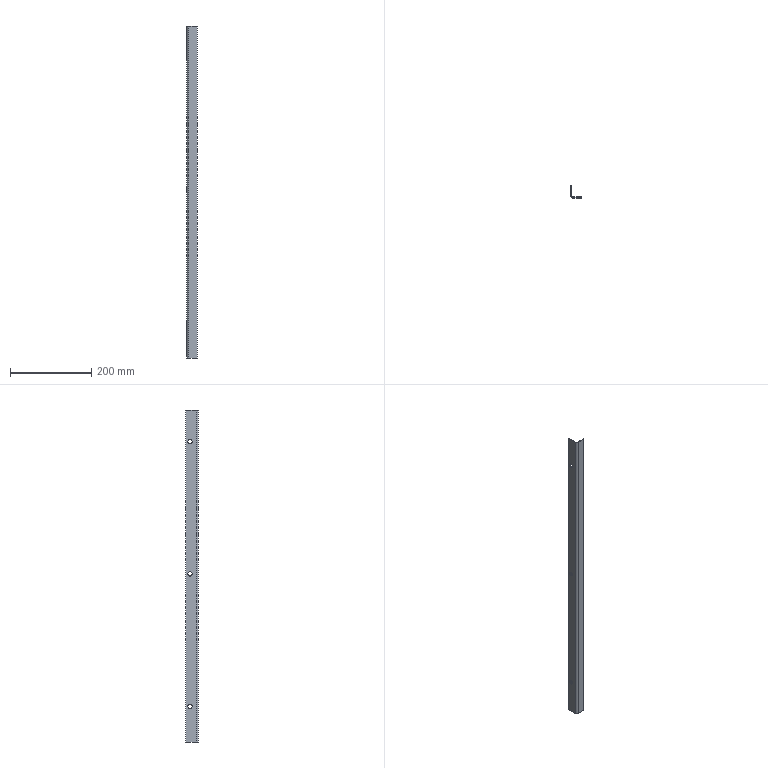Part | STEP file | 750038326 | 1 solid | 16 faces | box 25 x 30 x 815 mm | volume 103040 mm3 | cylinder 8 | plane 8 | commonest cylinder face diameters 10.5 x6 5 x1 10 x1
STEP:
#1=CARTESIAN_POINT('',(2.5,25.25,5.));
#2=VERTEX_POINT('',#1);
#3=CARTESIAN_POINT('',(2.5,14.75,5.));
#4=VERTEX_POINT('',#3);
#5=CARTESIAN_POINT('',(2.5,20.,5.));
#6=DIRECTION('',(-1.,0.,0.));
#7=DIRECTION('',(0.,-1.,0.));
#8=AXIS2_PLACEMENT_3D('',#5,#6,#7);
#9=CIRCLE('',#8,5.25);
#10=EDGE_CURVE('',#2,#4,#9,.T.);
#11=ORIENTED_EDGE('',*,*,#10,.F.);
#12=CARTESIAN_POINT('',(0.,25.25,5.));
#13=VERTEX_POINT('',#12);
#14=CARTESIAN_POINT('',(815.935,25.25,5.));
#15=DIRECTION('',(-1.,0.,0.));
#16=VECTOR('',#15,1000.);
#17=LINE('',#14,#16);
#18=EDGE_CURVE('',#2,#13,#17,.T.);
#19=ORIENTED_EDGE('',*,*,#18,.T.);
#20=CARTESIAN_POINT('',(0.,14.75,5.));
#21=VERTEX_POINT('',#20);
#22=CARTESIAN_POINT('',(0.,20.,5.));
#23=DIRECTION('',(1.,0.,0.));
#24=DIRECTION('',(0.,-1.,0.));
#25=AXIS2_PLACEMENT_3D('',#22,#23,#24);
#26=CIRCLE('',#25,5.25);
#27=EDGE_CURVE('',#21,#13,#26,.T.);
#28=ORIENTED_EDGE('',*,*,#27,.F.);
#29=CARTESIAN_POINT('',(815.935,14.75,5.));
#30=DIRECTION('',(-1.,0.,0.));
#31=VECTOR('',#30,1000.);
#32=LINE('',#29,#31);
#33=EDGE_CURVE('',#4,#21,#32,.T.);
#34=ORIENTED_EDGE('',*,*,#33,.F.);
#35=EDGE_LOOP('',(#11,#19,#28,#34));
#36=FACE_OUTER_BOUND('',#35,.T.);
#37=CARTESIAN_POINT('',(815.935,20.,5.));
#38=DIRECTION('',(-1.,0.,0.));
#39=DIRECTION('',(0.,-1.,0.));
#40=AXIS2_PLACEMENT_3D('',#37,#38,#39);
#41=CYLINDRICAL_SURFACE('',#40,5.25);
#42=ADVANCED_FACE('',(#36),#41,.F.);
#43=CARTESIAN_POINT('',(2.5,25.25,-320.));
#44=VERTEX_POINT('',#43);
#45=CARTESIAN_POINT('',(2.5,14.75,-320.));
#46=VERTEX_POINT('',#45);
#47=CARTESIAN_POINT('',(2.5,20.,-320.));
#48=DIRECTION('',(-1.,0.,0.));
#49=DIRECTION('',(0.,-1.,0.));
#50=AXIS2_PLACEMENT_3D('',#47,#48,#49);
#51=CIRCLE('',#50,5.25);
#52=EDGE_CURVE('',#44,#46,#51,.T.);
#53=ORIENTED_EDGE('',*,*,#52,.F.);
#54=CARTESIAN_POINT('',(0.,25.25,-320.));
#55=VERTEX_POINT('',#54);
#56=CARTESIAN_POINT('',(815.935,25.25,-320.));
#57=DIRECTION('',(-1.,0.,0.));
#58=VECTOR('',#57,1000.);
#59=LINE('',#56,#58);
#60=EDGE_CURVE('',#44,#55,#59,.T.);
#61=ORIENTED_EDGE('',*,*,#60,.T.);
#62=CARTESIAN_POINT('',(0.,14.75,-320.));
#63=VERTEX_POINT('',#62);
#64=CARTESIAN_POINT('',(0.,20.,-320.));
#65=DIRECTION('',(1.,0.,0.));
#66=DIRECTION('',(0.,-1.,0.));
#67=AXIS2_PLACEMENT_3D('',#64,#65,#66);
#68=CIRCLE('',#67,5.25);
#69=EDGE_CURVE('',#63,#55,#68,.T.);
#70=ORIENTED_EDGE('',*,*,#69,.F.);
#71=CARTESIAN_POINT('',(815.935,14.75,-320.));
#72=DIRECTION('',(-1.,0.,0.));
#73=VECTOR('',#72,1000.);
#74=LINE('',#71,#73);
#75=EDGE_CURVE('',#46,#63,#74,.T.);
#76=ORIENTED_EDGE('',*,*,#75,.F.);
#77=EDGE_LOOP('',(#53,#61,#70,#76));
#78=FACE_OUTER_BOUND('',#77,.T.);
#79=CARTESIAN_POINT('',(815.935,20.,-320.));
#80=DIRECTION('',(-1.,0.,0.));
#81=DIRECTION('',(0.,-1.,0.));
#82=AXIS2_PLACEMENT_3D('',#79,#80,#81);
#83=CYLINDRICAL_SURFACE('',#82,5.25);
#84=ADVANCED_FACE('',(#78),#83,.F.);
#85=CARTESIAN_POINT('',(2.5,25.25,330.));
#86=VERTEX_POINT('',#85);
#87=CARTESIAN_POINT('',(2.5,14.75,330.));
#88=VERTEX_POINT('',#87);
#89=CARTESIAN_POINT('',(2.5,20.,330.));
#90=DIRECTION('',(-1.,0.,0.));
#91=DIRECTION('',(0.,-1.,0.));
#92=AXIS2_PLACEMENT_3D('',#89,#90,#91);
#93=CIRCLE('',#92,5.25);
#94=EDGE_CURVE('',#86,#88,#93,.T.);
#95=ORIENTED_EDGE('',*,*,#94,.F.);
#96=CARTESIAN_POINT('',(0.,25.25,330.));
#97=VERTEX_POINT('',#96);
#98=CARTESIAN_POINT('',(815.935,25.25,330.));
#99=DIRECTION('',(-1.,0.,0.));
#100=VECTOR('',#99,1000.);
#101=LINE('',#98,#100);
#102=EDGE_CURVE('',#86,#97,#101,.T.);
#103=ORIENTED_EDGE('',*,*,#102,.T.);
#104=CARTESIAN_POINT('',(0.,14.75,330.));
#105=VERTEX_POINT('',#104);
#106=CARTESIAN_POINT('',(0.,20.,330.));
#107=DIRECTION('',(1.,0.,0.));
#108=DIRECTION('',(0.,-1.,0.));
#109=AXIS2_PLACEMENT_3D('',#106,#107,#108);
#110=CIRCLE('',#109,5.25);
#111=EDGE_CURVE('',#105,#97,#110,.T.);
#112=ORIENTED_EDGE('',*,*,#111,.F.);
#113=CARTESIAN_POINT('',(815.935,14.75,330.));
#114=DIRECTION('',(-1.,0.,0.));
#115=VECTOR('',#114,1000.);
#116=LINE('',#113,#115);
#117=EDGE_CURVE('',#88,#105,#116,.T.);
#118=ORIENTED_EDGE('',*,*,#117,.F.);
#119=EDGE_LOOP('',(#95,#103,#112,#118));
#120=FACE_OUTER_BOUND('',#119,.T.);
#121=CARTESIAN_POINT('',(815.935,20.,330.));
#122=DIRECTION('',(-1.,0.,0.));
#123=DIRECTION('',(0.,-1.,0.));
#124=AXIS2_PLACEMENT_3D('',#121,#122,#123);
#125=CYLINDRICAL_SURFACE('',#124,5.25);
#126=ADVANCED_FACE('',(#120),#125,.F.);
#127=CARTESIAN_POINT('',(0.,5.,407.5));
#128=VERTEX_POINT('',#127);
#129=CARTESIAN_POINT('',(0.,30.,407.5));
#130=VERTEX_POINT('',#129);
#131=CARTESIAN_POINT('',(0.,0.,407.5));
#132=DIRECTION('',(0.,1.,0.));
#133=VECTOR('',#132,1000.);
#134=LINE('',#131,#133);
#135=EDGE_CURVE('',#128,#130,#134,.T.);
#136=ORIENTED_EDGE('',*,*,#135,.T.);
#137=CARTESIAN_POINT('',(0.,30.,-407.5));
#138=VERTEX_POINT('',#137);
#139=CARTESIAN_POINT('',(0.,30.,407.5));
#140=DIRECTION('',(0.,0.,-1.));
#141=VECTOR('',#140,1000.);
#142=LINE('',#139,#141);
#143=EDGE_CURVE('',#130,#138,#142,.T.);
#144=ORIENTED_EDGE('',*,*,#143,.T.);
#145=CARTESIAN_POINT('',(0.,5.,-407.5));
#146=VERTEX_POINT('',#145);
#147=CARTESIAN_POINT('',(0.,0.,-407.5));
#148=DIRECTION('',(0.,-1.,0.));
#149=VECTOR('',#148,1000.);
#150=LINE('',#147,#149);
#151=EDGE_CURVE('',#138,#146,#150,.T.);
#152=ORIENTED_EDGE('',*,*,#151,.T.);
#153=CARTESIAN_POINT('',(0.,5.,407.5));
#154=DIRECTION('',(0.,0.,1.));
#155=VECTOR('',#154,1000.);
#156=LINE('',#153,#155);
#157=EDGE_CURVE('',#146,#128,#156,.T.);
#158=ORIENTED_EDGE('',*,*,#157,.T.);
#159=EDGE_LOOP('',(#136,#144,#152,#158));
#160=FACE_OUTER_BOUND('',#159,.T.);
#161=ORIENTED_EDGE('',*,*,#27,.T.);
#162=CARTESIAN_POINT('',(0.,20.,5.));
#163=DIRECTION('',(1.,0.,0.));
#164=DIRECTION('',(0.,-1.,0.));
#165=AXIS2_PLACEMENT_3D('',#162,#163,#164);
#166=CIRCLE('',#165,5.25);
#167=EDGE_CURVE('',#13,#21,#166,.T.);
#168=ORIENTED_EDGE('',*,*,#167,.T.);
#169=EDGE_LOOP('',(#161,#168));
#170=FACE_BOUND('',#169,.T.);
#171=ORIENTED_EDGE('',*,*,#69,.T.);
#172=CARTESIAN_POINT('',(0.,20.,-320.));
#173=DIRECTION('',(1.,0.,0.));
#174=DIRECTION('',(0.,-1.,0.));
#175=AXIS2_PLACEMENT_3D('',#172,#173,#174);
#176=CIRCLE('',#175,5.25);
#177=EDGE_CURVE('',#55,#63,#176,.T.);
#178=ORIENTED_EDGE('',*,*,#177,.T.);
#179=EDGE_LOOP('',(#171,#178));
#180=FACE_BOUND('',#179,.T.);
#181=ORIENTED_EDGE('',*,*,#111,.T.);
#182=CARTESIAN_POINT('',(0.,20.,330.));
#183=DIRECTION('',(1.,0.,0.));
#184=DIRECTION('',(0.,-1.,0.));
#185=AXIS2_PLACEMENT_3D('',#182,#183,#184);
#186=CIRCLE('',#185,5.25);
#187=EDGE_CURVE('',#97,#105,#186,.T.);
#188=ORIENTED_EDGE('',*,*,#187,.T.);
#189=EDGE_LOOP('',(#181,#188));
#190=FACE_BOUND('',#189,.T.);
#191=CARTESIAN_POINT('',(0.,0.,407.5));
#192=DIRECTION('',(-1.,0.,0.));
#193=DIRECTION('',(0.,-1.,0.));
#194=AXIS2_PLACEMENT_3D('',#191,#192,#193);
#195=PLANE('',#194);
#196=ADVANCED_FACE('',(#160,#170,#180,#190),#195,.T.);
#197=CARTESIAN_POINT('',(2.5,30.,-407.5));
#198=VERTEX_POINT('',#197);
#199=CARTESIAN_POINT('',(0.,30.,-407.5));
#200=DIRECTION('',(-1.,0.,0.));
#201=VECTOR('',#200,1000.);
#202=LINE('',#199,#201);
#203=EDGE_CURVE('',#198,#138,#202,.T.);
#204=ORIENTED_EDGE('',*,*,#203,.T.);
#205=ORIENTED_EDGE('',*,*,#143,.F.);
#206=CARTESIAN_POINT('',(2.5,30.,407.5));
#207=VERTEX_POINT('',#206);
#208=CARTESIAN_POINT('',(0.,30.,407.5));
#209=DIRECTION('',(1.,0.,0.));
#210=VECTOR('',#209,1000.);
#211=LINE('',#208,#210);
#212=EDGE_CURVE('',#130,#207,#211,.T.);
#213=ORIENTED_EDGE('',*,*,#212,.T.);
#214=CARTESIAN_POINT('',(2.5,30.,407.5));
#215=DIRECTION('',(0.,0.,-1.));
#216=VECTOR('',#215,1000.);
#217=LINE('',#214,#216);
#218=EDGE_CURVE('',#207,#198,#217,.T.);
#219=ORIENTED_EDGE('',*,*,#218,.T.);
#220=EDGE_LOOP('',(#204,#205,#213,#219));
#221=FACE_OUTER_BOUND('',#220,.T.);
#222=CARTESIAN_POINT('',(0.,30.,407.5));
#223=DIRECTION('',(0.,1.,0.));
#224=DIRECTION('',(-1.,0.,0.));
#225=AXIS2_PLACEMENT_3D('',#222,#223,#224);
#226=PLANE('',#225);
#227=ADVANCED_FACE('',(#221),#226,.T.);
#228=CARTESIAN_POINT('',(2.5,5.,407.5));
#229=VERTEX_POINT('',#228);
#230=CARTESIAN_POINT('',(2.5,0.,407.5));
#231=DIRECTION('',(0.,1.,0.));
#232=VECTOR('',#231,1000.);
#233=LINE('',#230,#232);
#234=EDGE_CURVE('',#229,#207,#233,.T.);
#235=ORIENTED_EDGE('',*,*,#234,.T.);
#236=ORIENTED_EDGE('',*,*,#212,.F.);
#237=ORIENTED_EDGE('',*,*,#135,.F.);
#238=CARTESIAN_POINT('',(5.,0.,407.5));
#239=VERTEX_POINT('',#238);
#240=CARTESIAN_POINT('',(5.,5.,407.5));
#241=DIRECTION('',(0.,0.,1.));
#242=DIRECTION('',(-1.,0.,0.));
#243=AXIS2_PLACEMENT_3D('',#240,#241,#242);
#244=CIRCLE('',#243,5.);
#245=EDGE_CURVE('',#128,#239,#244,.T.);
#246=ORIENTED_EDGE('',*,*,#245,.T.);
#247=CARTESIAN_POINT('',(25.,0.,407.5));
#248=VERTEX_POINT('',#247);
#249=CARTESIAN_POINT('',(0.,0.,407.5));
#250=DIRECTION('',(1.,0.,0.));
#251=VECTOR('',#250,1000.);
#252=LINE('',#249,#251);
#253=EDGE_CURVE('',#239,#248,#252,.T.);
#254=ORIENTED_EDGE('',*,*,#253,.T.);
#255=CARTESIAN_POINT('',(25.,2.5,407.5));
#256=VERTEX_POINT('',#255);
#257=CARTESIAN_POINT('',(25.,0.,407.5));
#258=DIRECTION('',(0.,1.,0.));
#259=VECTOR('',#258,1000.);
#260=LINE('',#257,#259);
#261=EDGE_CURVE('',#248,#256,#260,.T.);
#262=ORIENTED_EDGE('',*,*,#261,.T.);
#263=CARTESIAN_POINT('',(5.,2.5,407.5));
#264=VERTEX_POINT('',#263);
#265=CARTESIAN_POINT('',(0.,2.5,407.5));
#266=DIRECTION('',(-1.,0.,0.));
#267=VECTOR('',#266,1000.);
#268=LINE('',#265,#267);
#269=EDGE_CURVE('',#256,#264,#268,.T.);
#270=ORIENTED_EDGE('',*,*,#269,.T.);
#271=CARTESIAN_POINT('',(5.,5.,407.5));
#272=DIRECTION('',(0.,0.,-1.));
#273=DIRECTION('',(-1.,0.,0.));
#274=AXIS2_PLACEMENT_3D('',#271,#272,#273);
#275=CIRCLE('',#274,2.5);
#276=EDGE_CURVE('',#264,#229,#275,.T.);
#277=ORIENTED_EDGE('',*,*,#276,.T.);
#278=EDGE_LOOP('',(#235,#236,#237,#246,#254,#262,#270,#277));
#279=FACE_OUTER_BOUND('',#278,.T.);
#280=CARTESIAN_POINT('',(0.,0.,407.5));
#281=DIRECTION('',(0.,0.,1.));
#282=DIRECTION('',(1.,0.,0.));
#283=AXIS2_PLACEMENT_3D('',#280,#281,#282);
#284=PLANE('',#283);
#285=ADVANCED_FACE('',(#279),#284,.T.);
#286=ORIENTED_EDGE('',*,*,#245,.F.);
#287=ORIENTED_EDGE('',*,*,#157,.F.);
#288=CARTESIAN_POINT('',(5.,0.,-407.5));
#289=VERTEX_POINT('',#288);
#290=CARTESIAN_POINT('',(5.,5.,-407.5));
#291=DIRECTION('',(0.,0.,1.));
#292=DIRECTION('',(-1.,0.,0.));
#293=AXIS2_PLACEMENT_3D('',#290,#291,#292);
#294=CIRCLE('',#293,5.);
#295=EDGE_CURVE('',#146,#289,#294,.T.);
#296=ORIENTED_EDGE('',*,*,#295,.T.);
#297=CARTESIAN_POINT('',(5.,0.,407.5));
#298=DIRECTION('',(0.,0.,1.));
#299=VECTOR('',#298,1000.);
#300=LINE('',#297,#299);
#301=EDGE_CURVE('',#289,#239,#300,.T.);
#302=ORIENTED_EDGE('',*,*,#301,.T.);
#303=EDGE_LOOP('',(#286,#287,#296,#302));
#304=FACE_OUTER_BOUND('',#303,.T.);
#305=CARTESIAN_POINT('',(5.,5.,407.5));
#306=DIRECTION('',(0.,0.,-1.));
#307=DIRECTION('',(-1.,0.,0.));
#308=AXIS2_PLACEMENT_3D('',#305,#306,#307);
#309=CYLINDRICAL_SURFACE('',#308,5.);
#310=ADVANCED_FACE('',(#304),#309,.T.);
#311=ORIENTED_EDGE('',*,*,#295,.F.);
#312=ORIENTED_EDGE('',*,*,#151,.F.);
#313=ORIENTED_EDGE('',*,*,#203,.F.);
#314=CARTESIAN_POINT('',(2.5,5.,-407.5));
#315=VERTEX_POINT('',#314);
#316=CARTESIAN_POINT('',(2.5,0.,-407.5));
#317=DIRECTION('',(0.,1.,0.));
#318=VECTOR('',#317,1000.);
#319=LINE('',#316,#318);
#320=EDGE_CURVE('',#315,#198,#319,.T.);
#321=ORIENTED_EDGE('',*,*,#320,.F.);
#322=CARTESIAN_POINT('',(5.,2.5,-407.5));
#323=VERTEX_POINT('',#322);
#324=CARTESIAN_POINT('',(5.,5.,-407.5));
#325=DIRECTION('',(0.,0.,-1.));
#326=DIRECTION('',(-1.,0.,0.));
#327=AXIS2_PLACEMENT_3D('',#324,#325,#326);
#328=CIRCLE('',#327,2.5);
#329=EDGE_CURVE('',#323,#315,#328,.T.);
#330=ORIENTED_EDGE('',*,*,#329,.F.);
#331=CARTESIAN_POINT('',(25.,2.5,-407.5));
#332=VERTEX_POINT('',#331);
#333=CARTESIAN_POINT('',(25.,2.5,-407.5));
#334=DIRECTION('',(-1.,0.,0.));
#335=VECTOR('',#334,1000.);
#336=LINE('',#333,#335);
#337=EDGE_CURVE('',#332,#323,#336,.T.);
#338=ORIENTED_EDGE('',*,*,#337,.F.);
#339=CARTESIAN_POINT('',(25.,0.,-407.5));
#340=VERTEX_POINT('',#339);
#341=CARTESIAN_POINT('',(25.,0.,-407.5));
#342=DIRECTION('',(0.,1.,0.));
#343=VECTOR('',#342,1000.);
#344=LINE('',#341,#343);
#345=EDGE_CURVE('',#340,#332,#344,.T.);
#346=ORIENTED_EDGE('',*,*,#345,.F.);
#347=CARTESIAN_POINT('',(25.,0.,-407.5));
#348=DIRECTION('',(1.,0.,0.));
#349=VECTOR('',#348,1000.);
#350=LINE('',#347,#349);
#351=EDGE_CURVE('',#289,#340,#350,.T.);
#352=ORIENTED_EDGE('',*,*,#351,.F.);
#353=EDGE_LOOP('',(#311,#312,#313,#321,#330,#338,#346,#352));
#354=FACE_OUTER_BOUND('',#353,.T.);
#355=CARTESIAN_POINT('',(25.,0.,-407.5));
#356=DIRECTION('',(0.,0.,1.));
#357=DIRECTION('',(1.,0.,0.));
#358=AXIS2_PLACEMENT_3D('',#355,#356,#357);
#359=PLANE('',#358);
#360=ADVANCED_FACE('',(#354),#359,.F.);
#361=ORIENTED_EDGE('',*,*,#18,.F.);
#362=CARTESIAN_POINT('',(2.5,20.,5.));
#363=DIRECTION('',(-1.,0.,0.));
#364=DIRECTION('',(0.,-1.,0.));
#365=AXIS2_PLACEMENT_3D('',#362,#363,#364);
#366=CIRCLE('',#365,5.25);
#367=EDGE_CURVE('',#4,#2,#366,.T.);
#368=ORIENTED_EDGE('',*,*,#367,.F.);
#369=ORIENTED_EDGE('',*,*,#33,.T.);
#370=ORIENTED_EDGE('',*,*,#167,.F.);
#371=EDGE_LOOP('',(#361,#368,#369,#370));
#372=FACE_OUTER_BOUND('',#371,.T.);
#373=CARTESIAN_POINT('',(815.935,20.,5.));
#374=DIRECTION('',(-1.,0.,0.));
#375=DIRECTION('',(0.,-1.,0.));
#376=AXIS2_PLACEMENT_3D('',#373,#374,#375);
#377=CYLINDRICAL_SURFACE('',#376,5.25);
#378=ADVANCED_FACE('',(#372),#377,.F.);
#379=ORIENTED_EDGE('',*,*,#60,.F.);
#380=CARTESIAN_POINT('',(2.5,20.,-320.));
#381=DIRECTION('',(-1.,0.,0.));
#382=DIRECTION('',(0.,-1.,0.));
#383=AXIS2_PLACEMENT_3D('',#380,#381,#382);
#384=CIRCLE('',#383,5.25);
#385=EDGE_CURVE('',#46,#44,#384,.T.);
#386=ORIENTED_EDGE('',*,*,#385,.F.);
#387=ORIENTED_EDGE('',*,*,#75,.T.);
#388=ORIENTED_EDGE('',*,*,#177,.F.);
#389=EDGE_LOOP('',(#379,#386,#387,#388));
#390=FACE_OUTER_BOUND('',#389,.T.);
#391=CARTESIAN_POINT('',(815.935,20.,-320.));
#392=DIRECTION('',(-1.,0.,0.));
#393=DIRECTION('',(0.,-1.,0.));
#394=AXIS2_PLACEMENT_3D('',#391,#392,#393);
#395=CYLINDRICAL_SURFACE('',#394,5.25);
#396=ADVANCED_FACE('',(#390),#395,.F.);
#397=ORIENTED_EDGE('',*,*,#102,.F.);
#398=CARTESIAN_POINT('',(2.5,20.,330.));
#399=DIRECTION('',(-1.,0.,0.));
#400=DIRECTION('',(0.,-1.,0.));
#401=AXIS2_PLACEMENT_3D('',#398,#399,#400);
#402=CIRCLE('',#401,5.25);
#403=EDGE_CURVE('',#88,#86,#402,.T.);
#404=ORIENTED_EDGE('',*,*,#403,.F.);
#405=ORIENTED_EDGE('',*,*,#117,.T.);
#406=ORIENTED_EDGE('',*,*,#187,.F.);
#407=EDGE_LOOP('',(#397,#404,#405,#406));
#408=FACE_OUTER_BOUND('',#407,.T.);
#409=CARTESIAN_POINT('',(815.935,20.,330.));
#410=DIRECTION('',(-1.,0.,0.));
#411=DIRECTION('',(0.,-1.,0.));
#412=AXIS2_PLACEMENT_3D('',#409,#410,#411);
#413=CYLINDRICAL_SURFACE('',#412,5.25);
#414=ADVANCED_FACE('',(#408),#413,.F.);
#415=ORIENTED_EDGE('',*,*,#218,.F.);
#416=ORIENTED_EDGE('',*,*,#234,.F.);
#417=CARTESIAN_POINT('',(2.5,5.,407.5));
#418=DIRECTION('',(0.,0.,1.));
#419=VECTOR('',#418,1000.);
#420=LINE('',#417,#419);
#421=EDGE_CURVE('',#315,#229,#420,.T.);
#422=ORIENTED_EDGE('',*,*,#421,.F.);
#423=ORIENTED_EDGE('',*,*,#320,.T.);
#424=EDGE_LOOP('',(#415,#416,#422,#423));
#425=FACE_OUTER_BOUND('',#424,.T.);
#426=ORIENTED_EDGE('',*,*,#367,.T.);
#427=ORIENTED_EDGE('',*,*,#10,.T.);
#428=EDGE_LOOP('',(#426,#427));
#429=FACE_BOUND('',#428,.T.);
#430=ORIENTED_EDGE('',*,*,#385,.T.);
#431=ORIENTED_EDGE('',*,*,#52,.T.);
#432=EDGE_LOOP('',(#430,#431));
#433=FACE_BOUND('',#432,.T.);
#434=ORIENTED_EDGE('',*,*,#403,.T.);
#435=ORIENTED_EDGE('',*,*,#94,.T.);
#436=EDGE_LOOP('',(#434,#435));
#437=FACE_BOUND('',#436,.T.);
#438=CARTESIAN_POINT('',(2.5,0.,407.5));
#439=DIRECTION('',(-1.,0.,0.));
#440=DIRECTION('',(0.,-1.,0.));
#441=AXIS2_PLACEMENT_3D('',#438,#439,#440);
#442=PLANE('',#441);
#443=ADVANCED_FACE('',(#425,#429,#433,#437),#442,.F.);
#444=ORIENTED_EDGE('',*,*,#421,.T.);
#445=ORIENTED_EDGE('',*,*,#276,.F.);
#446=CARTESIAN_POINT('',(5.,2.5,407.5));
#447=DIRECTION('',(0.,0.,1.));
#448=VECTOR('',#447,1000.);
#449=LINE('',#446,#448);
#450=EDGE_CURVE('',#323,#264,#449,.T.);
#451=ORIENTED_EDGE('',*,*,#450,.F.);
#452=ORIENTED_EDGE('',*,*,#329,.T.);
#453=EDGE_LOOP('',(#444,#445,#451,#452));
#454=FACE_OUTER_BOUND('',#453,.T.);
#455=CARTESIAN_POINT('',(5.,5.,407.5));
#456=DIRECTION('',(0.,0.,-1.));
#457=DIRECTION('',(-1.,0.,0.));
#458=AXIS2_PLACEMENT_3D('',#455,#456,#457);
#459=CYLINDRICAL_SURFACE('',#458,2.5);
#460=ADVANCED_FACE('',(#454),#459,.F.);
#461=ORIENTED_EDGE('',*,*,#450,.T.);
#462=ORIENTED_EDGE('',*,*,#269,.F.);
#463=CARTESIAN_POINT('',(25.,2.5,407.5));
#464=DIRECTION('',(0.,0.,1.));
#465=VECTOR('',#464,1000.);
#466=LINE('',#463,#465);
#467=EDGE_CURVE('',#332,#256,#466,.T.);
#468=ORIENTED_EDGE('',*,*,#467,.F.);
#469=ORIENTED_EDGE('',*,*,#337,.T.);
#470=EDGE_LOOP('',(#461,#462,#468,#469));
#471=FACE_OUTER_BOUND('',#470,.T.);
#472=CARTESIAN_POINT('',(25.,2.5,407.5));
#473=DIRECTION('',(0.,-1.,0.));
#474=DIRECTION('',(0.,0.,-1.));
#475=AXIS2_PLACEMENT_3D('',#472,#473,#474);
#476=PLANE('',#475);
#477=ADVANCED_FACE('',(#471),#476,.F.);
#478=ORIENTED_EDGE('',*,*,#261,.F.);
#479=CARTESIAN_POINT('',(25.,0.,407.5));
#480=DIRECTION('',(0.,0.,1.));
#481=VECTOR('',#480,1000.);
#482=LINE('',#479,#481);
#483=EDGE_CURVE('',#340,#248,#482,.T.);
#484=ORIENTED_EDGE('',*,*,#483,.F.);
#485=ORIENTED_EDGE('',*,*,#345,.T.);
#486=ORIENTED_EDGE('',*,*,#467,.T.);
#487=EDGE_LOOP('',(#478,#484,#485,#486));
#488=FACE_OUTER_BOUND('',#487,.T.);
#489=CARTESIAN_POINT('',(25.,0.,407.5));
#490=DIRECTION('',(-1.,0.,0.));
#491=DIRECTION('',(0.,0.,1.));
#492=AXIS2_PLACEMENT_3D('',#489,#490,#491);
#493=PLANE('',#492);
#494=ADVANCED_FACE('',(#488),#493,.F.);
#495=ORIENTED_EDGE('',*,*,#253,.F.);
#496=ORIENTED_EDGE('',*,*,#301,.F.);
#497=ORIENTED_EDGE('',*,*,#351,.T.);
#498=ORIENTED_EDGE('',*,*,#483,.T.);
#499=EDGE_LOOP('',(#495,#496,#497,#498));
#500=FACE_OUTER_BOUND('',#499,.T.);
#501=CARTESIAN_POINT('',(25.,0.,407.5));
#502=DIRECTION('',(0.,-1.,0.));
#503=DIRECTION('',(0.,0.,-1.));
#504=AXIS2_PLACEMENT_3D('',#501,#502,#503);
#505=PLANE('',#504);
#506=ADVANCED_FACE('',(#500),#505,.T.);
#507=CLOSED_SHELL('',(#42,#84,#126,#196,#227,#285,#310,#360,#378,#396,#414,#443,#460,#477,#494,#506));
#508=MANIFOLD_SOLID_BREP('',#507);
#509=CARTESIAN_POINT('',(0.,0.,0.));
#510=DIRECTION('',(0.,0.,1.));
#511=DIRECTION('',(1.,0.,0.));
#512=AXIS2_PLACEMENT_3D('',#509,#510,#511);
#513=(LENGTH_UNIT()NAMED_UNIT(*)SI_UNIT(.MILLI.,.METRE.));
#514=UNCERTAINTY_MEASURE_WITH_UNIT(LENGTH_MEASURE(0.00001),#513,'','');
#515=(NAMED_UNIT(*)PLANE_ANGLE_UNIT()SI_UNIT($,.RADIAN.));
#516=(NAMED_UNIT(*)SI_UNIT($,.STERADIAN.)SOLID_ANGLE_UNIT());
#517=(GEOMETRIC_REPRESENTATION_CONTEXT(3)GLOBAL_UNCERTAINTY_ASSIGNED_CONTEXT((#514))GLOBAL_UNIT_ASSIGNED_CONTEXT((#513,#515,#516))REPRESENTATION_CONTEXT('',''));
#518=ADVANCED_BREP_SHAPE_REPRESENTATION('',(#508,#512),#517);